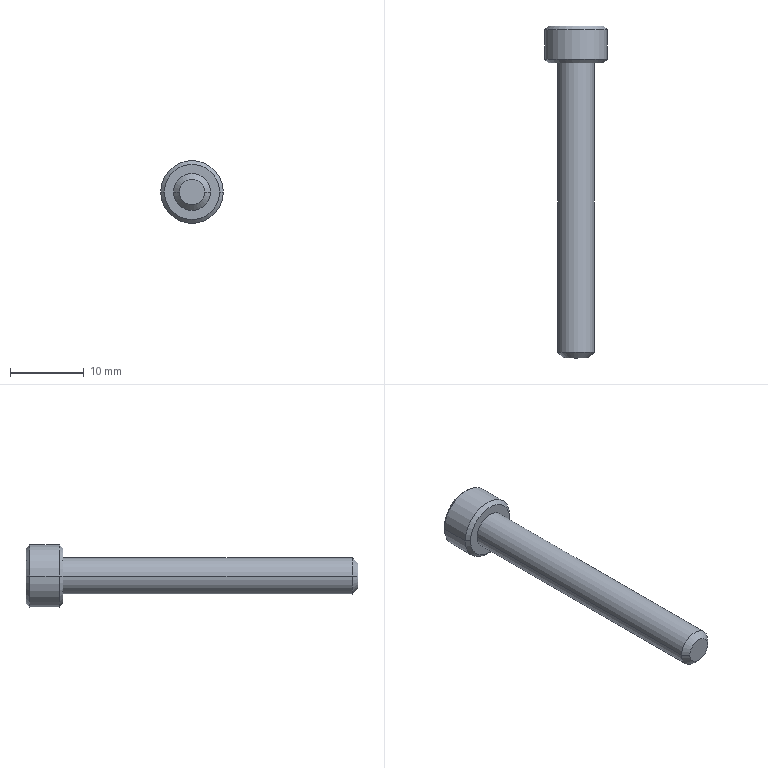Part | STEP file | BB62-M5-40L | 1 solid | 27 faces | box 8.5 x 45 x 8.5 mm | volume 1017 mm3 | plane 15 | cone 8 | cylinder 4 | commonest cylinder face diameters 5 x2 8.5 x2
STEP:
#1=CARTESIAN_POINT('',(0.,1.178,0.));
#2=VERTEX_POINT('',#1);
#3=CARTESIAN_POINT('',(2.29,2.5,0.));
#4=VERTEX_POINT('',#3);
#5=CARTESIAN_POINT('',(0.,1.178,0.));
#6=DIRECTION('',(0.866,0.5,0.));
#7=VECTOR('',#6,1000.);
#8=LINE('',#5,#7);
#9=EDGE_CURVE('',#2,#4,#8,.T.);
#10=ORIENTED_EDGE('',*,*,#9,.F.);
#11=CARTESIAN_POINT('',(-2.29,2.5,0.));
#12=VERTEX_POINT('',#11);
#13=CARTESIAN_POINT('',(0.,1.178,0.));
#14=DIRECTION('',(-0.866,0.5,0.));
#15=VECTOR('',#14,1000.);
#16=LINE('',#13,#15);
#17=EDGE_CURVE('',#2,#12,#16,.T.);
#18=ORIENTED_EDGE('',*,*,#17,.T.);
#19=CARTESIAN_POINT('',(-1.983,2.5,1.145));
#20=VERTEX_POINT('',#19);
#21=CARTESIAN_POINT('',(0.,2.5,0.));
#22=DIRECTION('',(0.,-1.,0.));
#23=DIRECTION('',(-1.,0.,0.));
#24=AXIS2_PLACEMENT_3D('',#21,#22,#23);
#25=CIRCLE('',#24,2.29);
#26=EDGE_CURVE('',#20,#12,#25,.T.);
#27=ORIENTED_EDGE('',*,*,#26,.F.);
#28=CARTESIAN_POINT('',(0.,2.5,2.29));
#29=VERTEX_POINT('',#28);
#30=CARTESIAN_POINT('',(0.,2.5,0.));
#31=DIRECTION('',(0.,-1.,0.));
#32=DIRECTION('',(-1.,0.,0.));
#33=AXIS2_PLACEMENT_3D('',#30,#31,#32);
#34=CIRCLE('',#33,2.29);
#35=EDGE_CURVE('',#29,#20,#34,.T.);
#36=ORIENTED_EDGE('',*,*,#35,.F.);
#37=CARTESIAN_POINT('',(1.983,2.5,1.145));
#38=VERTEX_POINT('',#37);
#39=CARTESIAN_POINT('',(0.,2.5,0.));
#40=DIRECTION('',(0.,-1.,0.));
#41=DIRECTION('',(-1.,0.,0.));
#42=AXIS2_PLACEMENT_3D('',#39,#40,#41);
#43=CIRCLE('',#42,2.29);
#44=EDGE_CURVE('',#38,#29,#43,.T.);
#45=ORIENTED_EDGE('',*,*,#44,.F.);
#46=CARTESIAN_POINT('',(0.,2.5,0.));
#47=DIRECTION('',(0.,-1.,0.));
#48=DIRECTION('',(-1.,0.,0.));
#49=AXIS2_PLACEMENT_3D('',#46,#47,#48);
#50=CIRCLE('',#49,2.29);
#51=EDGE_CURVE('',#4,#38,#50,.T.);
#52=ORIENTED_EDGE('',*,*,#51,.F.);
#53=EDGE_LOOP('',(#10,#18,#27,#36,#45,#52));
#54=FACE_OUTER_BOUND('',#53,.T.);
#55=CARTESIAN_POINT('',(0.,1001.178,0.));
#56=DIRECTION('',(0.,1.,0.));
#57=DIRECTION('',(1.,0.,0.));
#58=AXIS2_PLACEMENT_3D('',#55,#56,#57);
#59=CONICAL_SURFACE('',#58,1732.051,1.047);
#60=ADVANCED_FACE('',(#54),#59,.F.);
#61=CARTESIAN_POINT('',(1.7,-40.,0.));
#62=VERTEX_POINT('',#61);
#63=CARTESIAN_POINT('',(-1.7,-40.,0.));
#64=VERTEX_POINT('',#63);
#65=CARTESIAN_POINT('',(0.,-40.,0.));
#66=DIRECTION('',(0.,1.,0.));
#67=DIRECTION('',(1.,0.,0.));
#68=AXIS2_PLACEMENT_3D('',#65,#66,#67);
#69=CIRCLE('',#68,1.7);
#70=EDGE_CURVE('',#62,#64,#69,.T.);
#71=ORIENTED_EDGE('',*,*,#70,.T.);
#72=CARTESIAN_POINT('',(-2.5,-39.2,0.));
#73=VERTEX_POINT('',#72);
#74=CARTESIAN_POINT('',(-1.7,-40.,0.));
#75=DIRECTION('',(-0.7071,0.7071,0.));
#76=VECTOR('',#75,1000.);
#77=LINE('',#74,#76);
#78=EDGE_CURVE('',#64,#73,#77,.T.);
#79=ORIENTED_EDGE('',*,*,#78,.T.);
#80=CARTESIAN_POINT('',(2.5,-39.2,0.));
#81=VERTEX_POINT('',#80);
#82=CARTESIAN_POINT('',(0.,-39.2,0.));
#83=DIRECTION('',(0.,-1.,0.));
#84=DIRECTION('',(-1.,0.,0.));
#85=AXIS2_PLACEMENT_3D('',#82,#83,#84);
#86=CIRCLE('',#85,2.5);
#87=EDGE_CURVE('',#73,#81,#86,.T.);
#88=ORIENTED_EDGE('',*,*,#87,.T.);
#89=CARTESIAN_POINT('',(1.7,-40.,0.));
#90=DIRECTION('',(0.7071,0.7071,0.));
#91=VECTOR('',#90,1000.);
#92=LINE('',#89,#91);
#93=EDGE_CURVE('',#62,#81,#92,.T.);
#94=ORIENTED_EDGE('',*,*,#93,.F.);
#95=EDGE_LOOP('',(#71,#79,#88,#94));
#96=FACE_OUTER_BOUND('',#95,.T.);
#97=CARTESIAN_POINT('',(0.,-40.,0.));
#98=DIRECTION('',(0.,1.,0.));
#99=DIRECTION('',(1.,0.,0.));
#100=AXIS2_PLACEMENT_3D('',#97,#98,#99);
#101=CONICAL_SURFACE('',#100,1.7,0.7854);
#102=ADVANCED_FACE('',(#96),#101,.T.);
#103=ORIENTED_EDGE('',*,*,#87,.F.);
#104=CARTESIAN_POINT('',(-2.5,0.,0.));
#105=VERTEX_POINT('',#104);
#106=CARTESIAN_POINT('',(-2.5,-39.2,0.));
#107=DIRECTION('',(0.,1.,0.));
#108=VECTOR('',#107,1000.);
#109=LINE('',#106,#108);
#110=EDGE_CURVE('',#73,#105,#109,.T.);
#111=ORIENTED_EDGE('',*,*,#110,.T.);
#112=CARTESIAN_POINT('',(2.5,0.,0.));
#113=VERTEX_POINT('',#112);
#114=CARTESIAN_POINT('',(0.,0.,0.));
#115=DIRECTION('',(0.,-1.,0.));
#116=DIRECTION('',(-1.,0.,0.));
#117=AXIS2_PLACEMENT_3D('',#114,#115,#116);
#118=CIRCLE('',#117,2.5);
#119=EDGE_CURVE('',#105,#113,#118,.T.);
#120=ORIENTED_EDGE('',*,*,#119,.T.);
#121=CARTESIAN_POINT('',(2.5,-39.2,0.));
#122=DIRECTION('',(0.,1.,0.));
#123=VECTOR('',#122,1000.);
#124=LINE('',#121,#123);
#125=EDGE_CURVE('',#81,#113,#124,.T.);
#126=ORIENTED_EDGE('',*,*,#125,.F.);
#127=EDGE_LOOP('',(#103,#111,#120,#126));
#128=FACE_OUTER_BOUND('',#127,.T.);
#129=CARTESIAN_POINT('',(0.,-39.2,0.));
#130=DIRECTION('',(0.,1.,0.));
#131=DIRECTION('',(1.,0.,0.));
#132=AXIS2_PLACEMENT_3D('',#129,#130,#131);
#133=CYLINDRICAL_SURFACE('',#132,2.5);
#134=ADVANCED_FACE('',(#128),#133,.T.);
#135=CARTESIAN_POINT('',(-3.75,5.,0.));
#136=VERTEX_POINT('',#135);
#137=CARTESIAN_POINT('',(3.75,5.,0.));
#138=VERTEX_POINT('',#137);
#139=CARTESIAN_POINT('',(0.,5.,0.));
#140=DIRECTION('',(0.,-1.,0.));
#141=DIRECTION('',(-1.,0.,0.));
#142=AXIS2_PLACEMENT_3D('',#139,#140,#141);
#143=CIRCLE('',#142,3.75);
#144=EDGE_CURVE('',#136,#138,#143,.T.);
#145=ORIENTED_EDGE('',*,*,#144,.T.);
#146=CARTESIAN_POINT('',(4.25,4.5,0.));
#147=VERTEX_POINT('',#146);
#148=CARTESIAN_POINT('',(4.25,4.5,0.));
#149=DIRECTION('',(0.7071,-0.7071,0.));
#150=VECTOR('',#149,1000.);
#151=LINE('',#148,#150);
#152=EDGE_CURVE('',#138,#147,#151,.T.);
#153=ORIENTED_EDGE('',*,*,#152,.T.);
#154=CARTESIAN_POINT('',(-4.25,4.5,0.));
#155=VERTEX_POINT('',#154);
#156=CARTESIAN_POINT('',(0.,4.5,0.));
#157=DIRECTION('',(0.,-1.,0.));
#158=DIRECTION('',(-1.,0.,0.));
#159=AXIS2_PLACEMENT_3D('',#156,#157,#158);
#160=CIRCLE('',#159,4.25);
#161=EDGE_CURVE('',#155,#147,#160,.T.);
#162=ORIENTED_EDGE('',*,*,#161,.F.);
#163=CARTESIAN_POINT('',(-4.25,4.5,0.));
#164=DIRECTION('',(-0.7071,-0.7071,0.));
#165=VECTOR('',#164,1000.);
#166=LINE('',#163,#165);
#167=EDGE_CURVE('',#136,#155,#166,.T.);
#168=ORIENTED_EDGE('',*,*,#167,.F.);
#169=EDGE_LOOP('',(#145,#153,#162,#168));
#170=FACE_OUTER_BOUND('',#169,.T.);
#171=CARTESIAN_POINT('',(0.,4.5,0.));
#172=DIRECTION('',(0.,-1.,0.));
#173=DIRECTION('',(-1.,0.,0.));
#174=AXIS2_PLACEMENT_3D('',#171,#172,#173);
#175=CONICAL_SURFACE('',#174,4.25,0.7854);
#176=ADVANCED_FACE('',(#170),#175,.T.);
#177=ORIENTED_EDGE('',*,*,#161,.T.);
#178=CARTESIAN_POINT('',(4.25,0.5,0.));
#179=VERTEX_POINT('',#178);
#180=CARTESIAN_POINT('',(4.25,1.62,0.));
#181=DIRECTION('',(0.,-1.,0.));
#182=VECTOR('',#181,1000.);
#183=LINE('',#180,#182);
#184=EDGE_CURVE('',#147,#179,#183,.T.);
#185=ORIENTED_EDGE('',*,*,#184,.T.);
#186=CARTESIAN_POINT('',(-4.25,0.5,0.));
#187=VERTEX_POINT('',#186);
#188=CARTESIAN_POINT('',(0.,0.5,0.));
#189=DIRECTION('',(0.,-1.,0.));
#190=DIRECTION('',(-1.,0.,0.));
#191=AXIS2_PLACEMENT_3D('',#188,#189,#190);
#192=CIRCLE('',#191,4.25);
#193=EDGE_CURVE('',#187,#179,#192,.T.);
#194=ORIENTED_EDGE('',*,*,#193,.F.);
#195=CARTESIAN_POINT('',(-4.25,1.62,0.));
#196=DIRECTION('',(0.,-1.,0.));
#197=VECTOR('',#196,1000.);
#198=LINE('',#195,#197);
#199=EDGE_CURVE('',#155,#187,#198,.T.);
#200=ORIENTED_EDGE('',*,*,#199,.F.);
#201=EDGE_LOOP('',(#177,#185,#194,#200));
#202=FACE_OUTER_BOUND('',#201,.T.);
#203=CARTESIAN_POINT('',(0.,1.62,0.));
#204=DIRECTION('',(0.,-1.,0.));
#205=DIRECTION('',(-1.,0.,0.));
#206=AXIS2_PLACEMENT_3D('',#203,#204,#205);
#207=CYLINDRICAL_SURFACE('',#206,4.25);
#208=ADVANCED_FACE('',(#202),#207,.T.);
#209=CARTESIAN_POINT('',(-3.75,0.,0.));
#210=VERTEX_POINT('',#209);
#211=CARTESIAN_POINT('',(3.75,0.,0.));
#212=VERTEX_POINT('',#211);
#213=CARTESIAN_POINT('',(0.,0.,0.));
#214=DIRECTION('',(0.,-1.,0.));
#215=DIRECTION('',(-1.,0.,0.));
#216=AXIS2_PLACEMENT_3D('',#213,#214,#215);
#217=CIRCLE('',#216,3.75);
#218=EDGE_CURVE('',#210,#212,#217,.T.);
#219=ORIENTED_EDGE('',*,*,#218,.F.);
#220=CARTESIAN_POINT('',(-3.75,0.,0.));
#221=DIRECTION('',(-0.7071,0.7071,0.));
#222=VECTOR('',#221,1000.);
#223=LINE('',#220,#222);
#224=EDGE_CURVE('',#210,#187,#223,.T.);
#225=ORIENTED_EDGE('',*,*,#224,.T.);
#226=ORIENTED_EDGE('',*,*,#193,.T.);
#227=CARTESIAN_POINT('',(3.75,0.,0.));
#228=DIRECTION('',(0.7071,0.7071,0.));
#229=VECTOR('',#228,1000.);
#230=LINE('',#227,#229);
#231=EDGE_CURVE('',#212,#179,#230,.T.);
#232=ORIENTED_EDGE('',*,*,#231,.F.);
#233=EDGE_LOOP('',(#219,#225,#226,#232));
#234=FACE_OUTER_BOUND('',#233,.T.);
#235=CARTESIAN_POINT('',(0.,0.,0.));
#236=DIRECTION('',(0.,1.,0.));
#237=DIRECTION('',(1.,0.,0.));
#238=AXIS2_PLACEMENT_3D('',#235,#236,#237);
#239=CONICAL_SURFACE('',#238,3.75,0.7854);
#240=ADVANCED_FACE('',(#234),#239,.T.);
#241=ORIENTED_EDGE('',*,*,#144,.F.);
#242=CARTESIAN_POINT('',(0.,5.,0.));
#243=DIRECTION('',(0.,-1.,0.));
#244=DIRECTION('',(-1.,0.,0.));
#245=AXIS2_PLACEMENT_3D('',#242,#243,#244);
#246=CIRCLE('',#245,3.75);
#247=EDGE_CURVE('',#138,#136,#246,.T.);
#248=ORIENTED_EDGE('',*,*,#247,.F.);
#249=EDGE_LOOP('',(#241,#248));
#250=FACE_OUTER_BOUND('',#249,.T.);
#251=CARTESIAN_POINT('',(0.,5.,-2.29));
#252=VERTEX_POINT('',#251);
#253=CARTESIAN_POINT('',(-1.983,5.,-1.145));
#254=VERTEX_POINT('',#253);
#255=CARTESIAN_POINT('',(0.,5.,-2.29));
#256=DIRECTION('',(-0.866,0.,0.5));
#257=VECTOR('',#256,1000.);
#258=LINE('',#255,#257);
#259=EDGE_CURVE('',#252,#254,#258,.T.);
#260=ORIENTED_EDGE('',*,*,#259,.F.);
#261=CARTESIAN_POINT('',(1.983,5.,-1.145));
#262=VERTEX_POINT('',#261);
#263=CARTESIAN_POINT('',(1.983,5.,-1.145));
#264=DIRECTION('',(-0.866,0.,-0.5));
#265=VECTOR('',#264,1000.);
#266=LINE('',#263,#265);
#267=EDGE_CURVE('',#262,#252,#266,.T.);
#268=ORIENTED_EDGE('',*,*,#267,.F.);
#269=CARTESIAN_POINT('',(1.983,5.,1.145));
#270=VERTEX_POINT('',#269);
#271=CARTESIAN_POINT('',(1.983,5.,1.145));
#272=DIRECTION('',(0.,0.,-1.));
#273=VECTOR('',#272,1000.);
#274=LINE('',#271,#273);
#275=EDGE_CURVE('',#270,#262,#274,.T.);
#276=ORIENTED_EDGE('',*,*,#275,.F.);
#277=CARTESIAN_POINT('',(0.,5.,2.29));
#278=VERTEX_POINT('',#277);
#279=CARTESIAN_POINT('',(0.,5.,2.29));
#280=DIRECTION('',(0.866,0.,-0.5));
#281=VECTOR('',#280,1000.);
#282=LINE('',#279,#281);
#283=EDGE_CURVE('',#278,#270,#282,.T.);
#284=ORIENTED_EDGE('',*,*,#283,.F.);
#285=CARTESIAN_POINT('',(-1.983,5.,1.145));
#286=VERTEX_POINT('',#285);
#287=CARTESIAN_POINT('',(-1.983,5.,1.145));
#288=DIRECTION('',(0.866,0.,0.5));
#289=VECTOR('',#288,1000.);
#290=LINE('',#287,#289);
#291=EDGE_CURVE('',#286,#278,#290,.T.);
#292=ORIENTED_EDGE('',*,*,#291,.F.);
#293=CARTESIAN_POINT('',(-1.983,5.,-1.145));
#294=DIRECTION('',(0.,0.,1.));
#295=VECTOR('',#294,1000.);
#296=LINE('',#293,#295);
#297=EDGE_CURVE('',#254,#286,#296,.T.);
#298=ORIENTED_EDGE('',*,*,#297,.F.);
#299=EDGE_LOOP('',(#260,#268,#276,#284,#292,#298));
#300=FACE_BOUND('',#299,.T.);
#301=CARTESIAN_POINT('',(3.75,5.,0.));
#302=DIRECTION('',(0.,1.,0.));
#303=DIRECTION('',(1.,0.,0.));
#304=AXIS2_PLACEMENT_3D('',#301,#302,#303);
#305=PLANE('',#304);
#306=ADVANCED_FACE('',(#250,#300),#305,.T.);
#307=CARTESIAN_POINT('',(0.,0.,0.));
#308=DIRECTION('',(0.,-1.,0.));
#309=DIRECTION('',(-1.,0.,0.));
#310=AXIS2_PLACEMENT_3D('',#307,#308,#309);
#311=CIRCLE('',#310,2.5);
#312=EDGE_CURVE('',#113,#105,#311,.T.);
#313=ORIENTED_EDGE('',*,*,#312,.F.);
#314=ORIENTED_EDGE('',*,*,#119,.F.);
#315=EDGE_LOOP('',(#313,#314));
#316=FACE_BOUND('',#315,.T.);
#317=CARTESIAN_POINT('',(0.,0.,0.));
#318=DIRECTION('',(0.,-1.,0.));
#319=DIRECTION('',(-1.,0.,0.));
#320=AXIS2_PLACEMENT_3D('',#317,#318,#319);
#321=CIRCLE('',#320,3.75);
#322=EDGE_CURVE('',#212,#210,#321,.T.);
#323=ORIENTED_EDGE('',*,*,#322,.T.);
#324=ORIENTED_EDGE('',*,*,#218,.T.);
#325=EDGE_LOOP('',(#323,#324));
#326=FACE_OUTER_BOUND('',#325,.T.);
#327=CARTESIAN_POINT('',(0.,0.,0.));
#328=DIRECTION('',(0.,-1.,0.));
#329=DIRECTION('',(-1.,0.,0.));
#330=AXIS2_PLACEMENT_3D('',#327,#328,#329);
#331=PLANE('',#330);
#332=ADVANCED_FACE('',(#316,#326),#331,.T.);
#333=ORIENTED_EDGE('',*,*,#224,.F.);
#334=ORIENTED_EDGE('',*,*,#322,.F.);
#335=ORIENTED_EDGE('',*,*,#231,.T.);
#336=CARTESIAN_POINT('',(0.,0.5,0.));
#337=DIRECTION('',(0.,-1.,0.));
#338=DIRECTION('',(-1.,0.,0.));
#339=AXIS2_PLACEMENT_3D('',#336,#337,#338);
#340=CIRCLE('',#339,4.25);
#341=EDGE_CURVE('',#179,#187,#340,.T.);
#342=ORIENTED_EDGE('',*,*,#341,.T.);
#343=EDGE_LOOP('',(#333,#334,#335,#342));
#344=FACE_OUTER_BOUND('',#343,.T.);
#345=CARTESIAN_POINT('',(0.,0.,0.));
#346=DIRECTION('',(0.,1.,0.));
#347=DIRECTION('',(1.,0.,0.));
#348=AXIS2_PLACEMENT_3D('',#345,#346,#347);
#349=CONICAL_SURFACE('',#348,3.75,0.7854);
#350=ADVANCED_FACE('',(#344),#349,.T.);
#351=ORIENTED_EDGE('',*,*,#184,.F.);
#352=CARTESIAN_POINT('',(0.,4.5,0.));
#353=DIRECTION('',(0.,-1.,0.));
#354=DIRECTION('',(-1.,0.,0.));
#355=AXIS2_PLACEMENT_3D('',#352,#353,#354);
#356=CIRCLE('',#355,4.25);
#357=EDGE_CURVE('',#147,#155,#356,.T.);
#358=ORIENTED_EDGE('',*,*,#357,.T.);
#359=ORIENTED_EDGE('',*,*,#199,.T.);
#360=ORIENTED_EDGE('',*,*,#341,.F.);
#361=EDGE_LOOP('',(#351,#358,#359,#360));
#362=FACE_OUTER_BOUND('',#361,.T.);
#363=CARTESIAN_POINT('',(0.,1.62,0.));
#364=DIRECTION('',(0.,-1.,0.));
#365=DIRECTION('',(-1.,0.,0.));
#366=AXIS2_PLACEMENT_3D('',#363,#364,#365);
#367=CYLINDRICAL_SURFACE('',#366,4.25);
#368=ADVANCED_FACE('',(#362),#367,.T.);
#369=ORIENTED_EDGE('',*,*,#152,.F.);
#370=ORIENTED_EDGE('',*,*,#247,.T.);
#371=ORIENTED_EDGE('',*,*,#167,.T.);
#372=ORIENTED_EDGE('',*,*,#357,.F.);
#373=EDGE_LOOP('',(#369,#370,#371,#372));
#374=FACE_OUTER_BOUND('',#373,.T.);
#375=CARTESIAN_POINT('',(0.,4.5,0.));
#376=DIRECTION('',(0.,-1.,0.));
#377=DIRECTION('',(-1.,0.,0.));
#378=AXIS2_PLACEMENT_3D('',#375,#376,#377);
#379=CONICAL_SURFACE('',#378,4.25,0.7854);
#380=ADVANCED_FACE('',(#374),#379,.T.);
#381=ORIENTED_EDGE('',*,*,#110,.F.);
#382=CARTESIAN_POINT('',(0.,-39.2,0.));
#383=DIRECTION('',(0.,-1.,0.));
#384=DIRECTION('',(-1.,0.,0.));
#385=AXIS2_PLACEMENT_3D('',#382,#383,#384);
#386=CIRCLE('',#385,2.5);
#387=EDGE_CURVE('',#81,#73,#386,.T.);
#388=ORIENTED_EDGE('',*,*,#387,.F.);
#389=ORIENTED_EDGE('',*,*,#125,.T.);
#390=ORIENTED_EDGE('',*,*,#312,.T.);
#391=EDGE_LOOP('',(#381,#388,#389,#390));
#392=FACE_OUTER_BOUND('',#391,.T.);
#393=CARTESIAN_POINT('',(0.,-39.2,0.));
#394=DIRECTION('',(0.,1.,0.));
#395=DIRECTION('',(1.,0.,0.));
#396=AXIS2_PLACEMENT_3D('',#393,#394,#395);
#397=CYLINDRICAL_SURFACE('',#396,2.5);
#398=ADVANCED_FACE('',(#392),#397,.T.);
#399=ORIENTED_EDGE('',*,*,#70,.F.);
#400=CARTESIAN_POINT('',(0.,-40.,0.));
#401=DIRECTION('',(0.,1.,0.));
#402=DIRECTION('',(1.,0.,0.));
#403=AXIS2_PLACEMENT_3D('',#400,#401,#402);
#404=CIRCLE('',#403,1.7);
#405=EDGE_CURVE('',#64,#62,#404,.T.);
#406=ORIENTED_EDGE('',*,*,#405,.F.);
#407=EDGE_LOOP('',(#399,#406));
#408=FACE_OUTER_BOUND('',#407,.T.);
#409=CARTESIAN_POINT('',(0.,-40.,0.));
#410=DIRECTION('',(0.,-1.,0.));
#411=DIRECTION('',(-1.,0.,0.));
#412=AXIS2_PLACEMENT_3D('',#409,#410,#411);
#413=PLANE('',#412);
#414=ADVANCED_FACE('',(#408),#413,.T.);
#415=ORIENTED_EDGE('',*,*,#78,.F.);
#416=ORIENTED_EDGE('',*,*,#405,.T.);
#417=ORIENTED_EDGE('',*,*,#93,.T.);
#418=ORIENTED_EDGE('',*,*,#387,.T.);
#419=EDGE_LOOP('',(#415,#416,#417,#418));
#420=FACE_OUTER_BOUND('',#419,.T.);
#421=CARTESIAN_POINT('',(0.,-40.,0.));
#422=DIRECTION('',(0.,1.,0.));
#423=DIRECTION('',(1.,0.,0.));
#424=AXIS2_PLACEMENT_3D('',#421,#422,#423);
#425=CONICAL_SURFACE('',#424,1.7,0.7854);
#426=ADVANCED_FACE('',(#420),#425,.T.);
#427=CARTESIAN_POINT('',(1.983,2.5,-1.145));
#428=VERTEX_POINT('',#427);
#429=CARTESIAN_POINT('',(0.,2.5,-2.29));
#430=VERTEX_POINT('',#429);
#431=CARTESIAN_POINT('',(1.983,2.5,-1.145));
#432=DIRECTION('',(-0.866,0.,-0.5));
#433=VECTOR('',#432,1000.);
#434=LINE('',#431,#433);
#435=EDGE_CURVE('',#428,#430,#434,.T.);
#436=ORIENTED_EDGE('',*,*,#435,.F.);
#437=CARTESIAN_POINT('',(1.983,5.,-1.145));
#438=DIRECTION('',(0.,-1.,0.));
#439=VECTOR('',#438,1000.);
#440=LINE('',#437,#439);
#441=EDGE_CURVE('',#262,#428,#440,.T.);
#442=ORIENTED_EDGE('',*,*,#441,.F.);
#443=ORIENTED_EDGE('',*,*,#267,.T.);
#444=CARTESIAN_POINT('',(0.,5.,-2.29));
#445=DIRECTION('',(0.,-1.,0.));
#446=VECTOR('',#445,1000.);
#447=LINE('',#444,#446);
#448=EDGE_CURVE('',#252,#430,#447,.T.);
#449=ORIENTED_EDGE('',*,*,#448,.T.);
#450=EDGE_LOOP('',(#436,#442,#443,#449));
#451=FACE_OUTER_BOUND('',#450,.T.);
#452=CARTESIAN_POINT('',(1.983,5.,-1.145));
#453=DIRECTION('',(-0.5,0.,0.866));
#454=DIRECTION('',(0.866,0.,0.5));
#455=AXIS2_PLACEMENT_3D('',#452,#453,#454);
#456=PLANE('',#455);
#457=ADVANCED_FACE('',(#451),#456,.T.);
#458=CARTESIAN_POINT('',(-1.983,2.5,-1.145));
#459=VERTEX_POINT('',#458);
#460=CARTESIAN_POINT('',(0.,2.5,-2.29));
#461=DIRECTION('',(-0.866,0.,0.5));
#462=VECTOR('',#461,1000.);
#463=LINE('',#460,#462);
#464=EDGE_CURVE('',#430,#459,#463,.T.);
#465=ORIENTED_EDGE('',*,*,#464,.F.);
#466=ORIENTED_EDGE('',*,*,#448,.F.);
#467=ORIENTED_EDGE('',*,*,#259,.T.);
#468=CARTESIAN_POINT('',(-1.983,5.,-1.145));
#469=DIRECTION('',(0.,-1.,0.));
#470=VECTOR('',#469,1000.);
#471=LINE('',#468,#470);
#472=EDGE_CURVE('',#254,#459,#471,.T.);
#473=ORIENTED_EDGE('',*,*,#472,.T.);
#474=EDGE_LOOP('',(#465,#466,#467,#473));
#475=FACE_OUTER_BOUND('',#474,.T.);
#476=CARTESIAN_POINT('',(0.,5.,-2.29));
#477=DIRECTION('',(0.5,0.,0.866));
#478=DIRECTION('',(0.866,0.,-0.5));
#479=AXIS2_PLACEMENT_3D('',#476,#477,#478);
#480=PLANE('',#479);
#481=ADVANCED_FACE('',(#475),#480,.T.);
#482=CARTESIAN_POINT('',(-1.983,2.5,-1.145));
#483=DIRECTION('',(0.,0.,1.));
#484=VECTOR('',#483,1000.);
#485=LINE('',#482,#484);
#486=EDGE_CURVE('',#459,#20,#485,.T.);
#487=ORIENTED_EDGE('',*,*,#486,.F.);
#488=ORIENTED_EDGE('',*,*,#472,.F.);
#489=ORIENTED_EDGE('',*,*,#297,.T.);
#490=CARTESIAN_POINT('',(-1.983,5.,1.145));
#491=DIRECTION('',(0.,-1.,0.));
#492=VECTOR('',#491,1000.);
#493=LINE('',#490,#492);
#494=EDGE_CURVE('',#286,#20,#493,.T.);
#495=ORIENTED_EDGE('',*,*,#494,.T.);
#496=EDGE_LOOP('',(#487,#488,#489,#495));
#497=FACE_OUTER_BOUND('',#496,.T.);
#498=CARTESIAN_POINT('',(-1.983,5.,-1.145));
#499=DIRECTION('',(1.,0.,0.));
#500=DIRECTION('',(0.,0.,-1.));
#501=AXIS2_PLACEMENT_3D('',#498,#499,#500);
#502=PLANE('',#501);
#503=ADVANCED_FACE('',(#497),#502,.T.);
#504=CARTESIAN_POINT('',(-1.983,2.5,1.145));
#505=DIRECTION('',(0.866,0.,0.5));
#506=VECTOR('',#505,1000.);
#507=LINE('',#504,#506);
#508=EDGE_CURVE('',#20,#29,#507,.T.);
#509=ORIENTED_EDGE('',*,*,#508,.F.);
#510=ORIENTED_EDGE('',*,*,#494,.F.);
#511=ORIENTED_EDGE('',*,*,#291,.T.);
#512=CARTESIAN_POINT('',(0.,5.,2.29));
#513=DIRECTION('',(0.,-1.,0.));
#514=VECTOR('',#513,1000.);
#515=LINE('',#512,#514);
#516=EDGE_CURVE('',#278,#29,#515,.T.);
#517=ORIENTED_EDGE('',*,*,#516,.T.);
#518=EDGE_LOOP('',(#509,#510,#511,#517));
#519=FACE_OUTER_BOUND('',#518,.T.);
#520=CARTESIAN_POINT('',(-1.983,5.,1.145));
#521=DIRECTION('',(0.5,0.,-0.866));
#522=DIRECTION('',(-0.866,0.,-0.5));
#523=AXIS2_PLACEMENT_3D('',#520,#521,#522);
#524=PLANE('',#523);
#525=ADVANCED_FACE('',(#519),#524,.T.);
#526=CARTESIAN_POINT('',(0.,2.5,2.29));
#527=DIRECTION('',(0.866,0.,-0.5));
#528=VECTOR('',#527,1000.);
#529=LINE('',#526,#528);
#530=EDGE_CURVE('',#29,#38,#529,.T.);
#531=ORIENTED_EDGE('',*,*,#530,.F.);
#532=ORIENTED_EDGE('',*,*,#516,.F.);
#533=ORIENTED_EDGE('',*,*,#283,.T.);
#534=CARTESIAN_POINT('',(1.983,5.,1.145));
#535=DIRECTION('',(0.,-1.,0.));
#536=VECTOR('',#535,1000.);
#537=LINE('',#534,#536);
#538=EDGE_CURVE('',#270,#38,#537,.T.);
#539=ORIENTED_EDGE('',*,*,#538,.T.);
#540=EDGE_LOOP('',(#531,#532,#533,#539));
#541=FACE_OUTER_BOUND('',#540,.T.);
#542=CARTESIAN_POINT('',(0.,5.,2.29));
#543=DIRECTION('',(-0.5,0.,-0.866));
#544=DIRECTION('',(-0.866,0.,0.5));
#545=AXIS2_PLACEMENT_3D('',#542,#543,#544);
#546=PLANE('',#545);
#547=ADVANCED_FACE('',(#541),#546,.T.);
#548=CARTESIAN_POINT('',(1.983,2.5,1.145));
#549=DIRECTION('',(0.,0.,-1.));
#550=VECTOR('',#549,1000.);
#551=LINE('',#548,#550);
#552=EDGE_CURVE('',#38,#428,#551,.T.);
#553=ORIENTED_EDGE('',*,*,#552,.F.);
#554=ORIENTED_EDGE('',*,*,#538,.F.);
#555=ORIENTED_EDGE('',*,*,#275,.T.);
#556=ORIENTED_EDGE('',*,*,#441,.T.);
#557=EDGE_LOOP('',(#553,#554,#555,#556));
#558=FACE_OUTER_BOUND('',#557,.T.);
#559=CARTESIAN_POINT('',(1.983,5.,1.145));
#560=DIRECTION('',(-1.,0.,0.));
#561=DIRECTION('',(0.,0.,1.));
#562=AXIS2_PLACEMENT_3D('',#559,#560,#561);
#563=PLANE('',#562);
#564=ADVANCED_FACE('',(#558),#563,.T.);
#565=ORIENTED_EDGE('',*,*,#435,.T.);
#566=CARTESIAN_POINT('',(0.,2.5,0.));
#567=DIRECTION('',(0.,-1.,0.));
#568=DIRECTION('',(-1.,0.,0.));
#569=AXIS2_PLACEMENT_3D('',#566,#567,#568);
#570=CIRCLE('',#569,2.29);
#571=EDGE_CURVE('',#430,#428,#570,.T.);
#572=ORIENTED_EDGE('',*,*,#571,.T.);
#573=EDGE_LOOP('',(#565,#572));
#574=FACE_OUTER_BOUND('',#573,.T.);
#575=CARTESIAN_POINT('',(0.,2.5,0.));
#576=DIRECTION('',(0.,1.,0.));
#577=DIRECTION('',(1.,0.,0.));
#578=AXIS2_PLACEMENT_3D('',#575,#576,#577);
#579=PLANE('',#578);
#580=ADVANCED_FACE('',(#574),#579,.F.);
#581=ORIENTED_EDGE('',*,*,#552,.T.);
#582=CARTESIAN_POINT('',(0.,2.5,0.));
#583=DIRECTION('',(0.,-1.,0.));
#584=DIRECTION('',(-1.,0.,0.));
#585=AXIS2_PLACEMENT_3D('',#582,#583,#584);
#586=CIRCLE('',#585,2.29);
#587=EDGE_CURVE('',#428,#4,#586,.T.);
#588=ORIENTED_EDGE('',*,*,#587,.T.);
#589=ORIENTED_EDGE('',*,*,#51,.T.);
#590=EDGE_LOOP('',(#581,#588,#589));
#591=FACE_OUTER_BOUND('',#590,.T.);
#592=CARTESIAN_POINT('',(0.,2.5,0.));
#593=DIRECTION('',(0.,1.,0.));
#594=DIRECTION('',(1.,0.,0.));
#595=AXIS2_PLACEMENT_3D('',#592,#593,#594);
#596=PLANE('',#595);
#597=ADVANCED_FACE('',(#591),#596,.F.);
#598=ORIENTED_EDGE('',*,*,#530,.T.);
#599=ORIENTED_EDGE('',*,*,#44,.T.);
#600=EDGE_LOOP('',(#598,#599));
#601=FACE_OUTER_BOUND('',#600,.T.);
#602=CARTESIAN_POINT('',(0.,2.5,0.));
#603=DIRECTION('',(0.,1.,0.));
#604=DIRECTION('',(1.,0.,0.));
#605=AXIS2_PLACEMENT_3D('',#602,#603,#604);
#606=PLANE('',#605);
#607=ADVANCED_FACE('',(#601),#606,.F.);
#608=ORIENTED_EDGE('',*,*,#508,.T.);
#609=ORIENTED_EDGE('',*,*,#35,.T.);
#610=EDGE_LOOP('',(#608,#609));
#611=FACE_OUTER_BOUND('',#610,.T.);
#612=CARTESIAN_POINT('',(0.,2.5,0.));
#613=DIRECTION('',(0.,1.,0.));
#614=DIRECTION('',(1.,0.,0.));
#615=AXIS2_PLACEMENT_3D('',#612,#613,#614);
#616=PLANE('',#615);
#617=ADVANCED_FACE('',(#611),#616,.F.);
#618=ORIENTED_EDGE('',*,*,#486,.T.);
#619=ORIENTED_EDGE('',*,*,#26,.T.);
#620=CARTESIAN_POINT('',(0.,2.5,0.));
#621=DIRECTION('',(0.,-1.,0.));
#622=DIRECTION('',(-1.,0.,0.));
#623=AXIS2_PLACEMENT_3D('',#620,#621,#622);
#624=CIRCLE('',#623,2.29);
#625=EDGE_CURVE('',#12,#459,#624,.T.);
#626=ORIENTED_EDGE('',*,*,#625,.T.);
#627=EDGE_LOOP('',(#618,#619,#626));
#628=FACE_OUTER_BOUND('',#627,.T.);
#629=CARTESIAN_POINT('',(0.,2.5,0.));
#630=DIRECTION('',(0.,1.,0.));
#631=DIRECTION('',(1.,0.,0.));
#632=AXIS2_PLACEMENT_3D('',#629,#630,#631);
#633=PLANE('',#632);
#634=ADVANCED_FACE('',(#628),#633,.F.);
#635=ORIENTED_EDGE('',*,*,#464,.T.);
#636=CARTESIAN_POINT('',(0.,2.5,0.));
#637=DIRECTION('',(0.,-1.,0.));
#638=DIRECTION('',(-1.,0.,0.));
#639=AXIS2_PLACEMENT_3D('',#636,#637,#638);
#640=CIRCLE('',#639,2.29);
#641=EDGE_CURVE('',#459,#430,#640,.T.);
#642=ORIENTED_EDGE('',*,*,#641,.T.);
#643=EDGE_LOOP('',(#635,#642));
#644=FACE_OUTER_BOUND('',#643,.T.);
#645=CARTESIAN_POINT('',(0.,2.5,0.));
#646=DIRECTION('',(0.,1.,0.));
#647=DIRECTION('',(1.,0.,0.));
#648=AXIS2_PLACEMENT_3D('',#645,#646,#647);
#649=PLANE('',#648);
#650=ADVANCED_FACE('',(#644),#649,.F.);
#651=ORIENTED_EDGE('',*,*,#17,.F.);
#652=ORIENTED_EDGE('',*,*,#9,.T.);
#653=ORIENTED_EDGE('',*,*,#587,.F.);
#654=ORIENTED_EDGE('',*,*,#571,.F.);
#655=ORIENTED_EDGE('',*,*,#641,.F.);
#656=ORIENTED_EDGE('',*,*,#625,.F.);
#657=EDGE_LOOP('',(#651,#652,#653,#654,#655,#656));
#658=FACE_OUTER_BOUND('',#657,.T.);
#659=CARTESIAN_POINT('',(0.,1001.178,0.));
#660=DIRECTION('',(0.,1.,0.));
#661=DIRECTION('',(1.,0.,0.));
#662=AXIS2_PLACEMENT_3D('',#659,#660,#661);
#663=CONICAL_SURFACE('',#662,1732.051,1.047);
#664=ADVANCED_FACE('',(#658),#663,.F.);
#665=CLOSED_SHELL('',(#60,#102,#134,#176,#208,#240,#306,#332,#350,#368,#380,#398,#414,#426,#457,#481,#503,#525,#547,#564,#580,#597,#607,#617,#634,#650,#664));
#666=MANIFOLD_SOLID_BREP('',#665);
#667=CARTESIAN_POINT('',(0.,0.,0.));
#668=DIRECTION('',(0.,0.,1.));
#669=DIRECTION('',(1.,0.,0.));
#670=AXIS2_PLACEMENT_3D('',#667,#668,#669);
#671=(LENGTH_UNIT()NAMED_UNIT(*)SI_UNIT(.MILLI.,.METRE.));
#672=UNCERTAINTY_MEASURE_WITH_UNIT(LENGTH_MEASURE(0.00001),#671,'','');
#673=(NAMED_UNIT(*)PLANE_ANGLE_UNIT()SI_UNIT($,.RADIAN.));
#674=(NAMED_UNIT(*)SI_UNIT($,.STERADIAN.)SOLID_ANGLE_UNIT());
#675=(GEOMETRIC_REPRESENTATION_CONTEXT(3)GLOBAL_UNCERTAINTY_ASSIGNED_CONTEXT((#672))GLOBAL_UNIT_ASSIGNED_CONTEXT((#671,#673,#674))REPRESENTATION_CONTEXT('',''));
#676=ADVANCED_BREP_SHAPE_REPRESENTATION('',(#666,#670),#675);